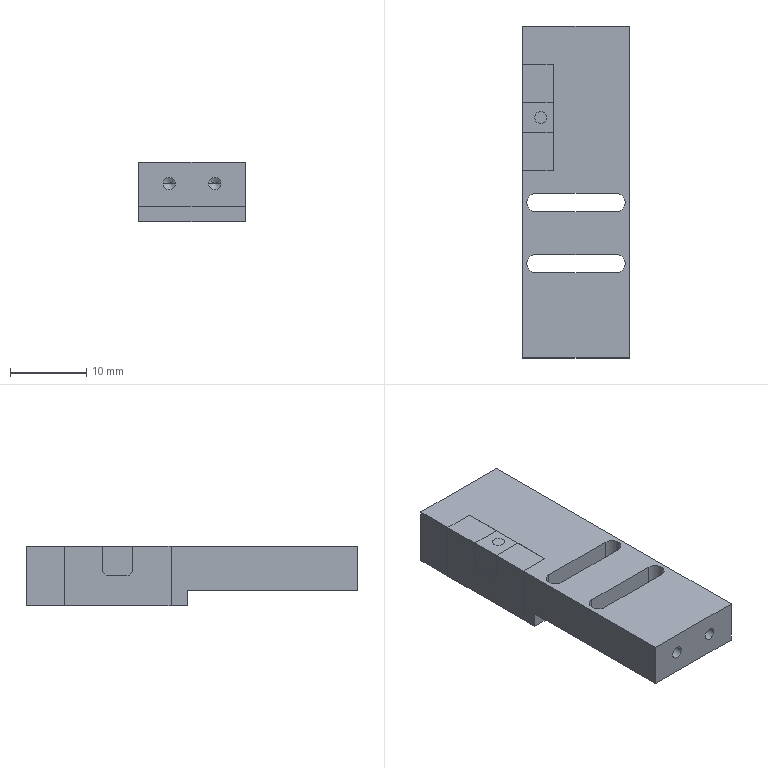NC program | NX | posted with a generic post | part box 14 x 43.5 x 7.8 mm
Whole program:
N10 G17 G21 G94 G90
(DRILLING_COPY_1_COPY , TOOL : D6A45)
N12 T07 M6
N14 G54
N16 G17 G0 G90 X-14.25 Y0.4 B0. C0. S5000 M3
N18 G43 Z30. H7
N20 G94 G81 G98 Z-1. F250. R3.
N22 X-5.25
N24 G80
N26 G0 X-5.25 Y0.4 Z30.
N28 M5
(DRILLING_COPY_COPY_COPY_COPY , TOOL : 1.6ZT)
N30 T14 M6
N32 G54
N34 G17 G0 G90 X-14.25 Y0.4 B0. C0. S2000 M3
N36 G43 Z30. H14
N38 G94 G83 G98 Z-9.681 F150. Q2. R3.
N40 X-5.25
N42 G80
N44 G0 X-5.25 Y0.4 Z30.
N46 M5
(FLOOR_WALL_1_COPY_1 , TOOL : D4)
N48 T04 M6
N50 G54
N52 G17 G0 G90 X-9.75 Y-7.9 B0. C0. S9500 M3
N54 G43 Z30. H4
N56 Z0.61
N58 G94 G1 Z-0.39 F1000.
N60 Y-3.9
N62 X-14.65 F2500.
N64 Y3.9
N66 X-13.85
N68 Y-0.27
N70 X-12.12 Y-2.
N72 X-7.38
N74 X-5.65 Y-0.27
N76 Y3.9
N78 X-4.85
N80 Y-3.9
N82 X-9.75
N84 Y-7.9
N86 Z0.61
N88 G0 Z0.22
N90 G1 Z-0.78 F1000.
N92 Y-3.9
N94 X-14.65 F2500.
N96 Y3.9
N98 X-13.85
N100 Y-0.27
N102 X-12.12 Y-2.
N104 X-7.38
N106 X-5.65 Y-0.27
N108 Y3.9
N110 X-4.85
N112 Y-3.9
N114 X-9.75
N116 Y-7.9
N118 Z0.22
N120 G0 Z-0.17
N122 G1 Z-1.17 F1000.
N124 Y-3.9
N126 X-14.65 F2500.
N128 Y3.9
N130 X-13.85
N132 Y-0.27
N134 X-12.12 Y-2.
N136 X-7.38
N138 X-5.65 Y-0.27
N140 Y3.9
N142 X-4.85
N144 Y-3.9
N146 X-9.75
N148 Y-7.9
N150 Z-0.17
N152 G0 Z-0.56
N154 G1 Z-1.56 F1000.
N156 Y-3.9
N158 X-14.65 F2500.
N160 Y3.9
N162 X-13.85
N164 Y-0.27
N166 X-12.12 Y-2.
N168 X-7.38
N170 X-5.65 Y-0.27
N172 Y3.9
N174 X-4.85
N176 Y-3.9
N178 X-9.75
N180 Y-7.9
N182 Z-0.56
N184 G0 Z-0.95
N186 G1 Z-1.95 F1000.
N188 Y-3.9
N190 X-14.65 F2500.
N192 Y3.9
N194 X-13.85
N196 Y-0.27
N198 X-12.12 Y-2.
N200 X-7.38
N202 X-5.65 Y-0.27
N204 Y3.9
N206 X-4.85
N208 Y-3.9
N210 X-9.75
N212 Y-7.9
N214 Z-0.95
N216 G0 Z-1.34
N218 G1 Z-2.34 F1000.
N220 Y-3.9
N222 X-14.65 F2500.
N224 Y3.9
N226 X-13.85
N228 Y-0.27
N230 X-12.12 Y-2.
N232 X-7.38
N234 X-5.65 Y-0.27
N236 Y3.9
N238 X-4.85
N240 Y-3.9
N242 X-9.75
N244 Y-7.9
N246 Z-1.34
N248 G0 Z-1.73
N250 G1 Z-2.73 F1000.
N252 Y-3.9
N254 X-14.65 F2500.
N256 Y3.9
N258 X-13.85
N260 Y-0.27
N262 X-12.12 Y-2.
N264 X-7.38
N266 X-5.65 Y-0.27
N268 Y3.9
N270 X-4.85
N272 Y-3.9
N274 X-9.75
N276 Y-7.9
N278 Z-1.73
N280 G0 Z-2.12
N282 G1 Z-3.12 F1000.
N284 Y-3.9
N286 X-14.65 F2500.
N288 Y3.9
N290 X-13.85
N292 Y-0.27
N294 X-12.12 Y-2.
N296 X-7.38
N298 X-5.65 Y-0.27
N300 Y3.9
N302 X-4.85
N304 Y-3.9
N306 X-9.75
N308 Y-7.9
N310 Z-2.12
N312 G0 Z-2.51
N314 G1 Z-3.51 F1000.
N316 Y-3.9
N318 X-14.65 F2500.
N320 Y3.9
N322 X-13.85
N324 Y-0.27
N326 X-12.12 Y-2.
N328 X-7.38
N330 X-5.65 Y-0.27
N332 Y3.9
N334 X-4.85
N336 Y-3.9
N338 X-9.75
N340 Y-7.9
N342 Z-2.51
N344 G0 Z-2.9
N346 G1 Z-3.9 F1000.
N348 Y-3.9
N350 X-14.65 F2500.
N352 Y3.9
N354 X-13.85
N356 Y-0.27
N358 X-12.12 Y-2.
N360 X-7.38
N362 X-5.65 Y-0.27
N364 Y3.9
N366 X-4.85
N368 Y-3.9
N370 X-9.75
N372 Y-7.9
N374 Z-2.9
N376 G0 Z30.
(FLOOR_WALL_1_COPY_COPY , TOOL : D4)
N378 X-14.449 Y-8.
N380 Z-3.
N382 G1 Z-4. F1000.
N384 Y-5.9
N386 Y5.9 F1200.
N388 X-14.05
N390 Y-0.27
N392 X-14.053 Y-0.324
N394 X-14.032 Y-0.375
N396 X-13.991 Y-0.411
N398 X-12.569 Y-1.833
N400 Y-5.9
N402 X-10.689
N404 Y-2.2
N406 X-8.81
N408 Y-5.9
N410 X-6.93
N412 Y-1.832
N414 X-5.509 Y-0.411
N416 X-5.468 Y-0.375
N418 X-5.447 Y-0.324
N420 X-5.45 Y-0.27
N422 Y5.9
N424 X-5.05
N426 Y-5.9
N428 Y-8.
N430 Z-3.
N432 G0 X-4.85
N434 G1 Z-4. F1000.
N436 Y-5.9
N438 Y5.9 F1200.
N440 Y8.
N442 X-5.65
N444 Y5.9 F1000.
N446 Y-0.27 F1200.
N448 X-7.38 Y-2.
N450 X-12.12
N452 X-13.85 Y-0.27
N454 Y5.9
N456 Y8.
N458 X-14.65
N460 Y5.9 F1000.
N462 Y-5.9 F1200.
N464 Y-8.
N466 Z-3.
N468 G0 Z30.
N470 M5
(PLANAR_MILL_COPY_1_COPY_COPY_1 , TOOL : D6A45)
N472 T07 M6
N474 G54
N476 G17 G0 G90 X-4.92 Y-1.8 B0. C0. S9500 M3
N478 G43 Z30. H7
N480 Z0.5
N482 G94 G1 Z-1. F1250.
N484 X-4.516 Y-2.5
N486 G3 X-3.65 Y-3. R1.
N488 G1 Y3.
N490 X-6.85
N492 Y0.641
N494 G2 X-7.143 Y-0.066 R1.
N496 G1 X-7.584 Y-0.507
N498 G2 X-8.291 Y-0.8 R1.
N500 G1 X-11.209
N502 G2 X-11.916 Y-0.507 R1.
N504 G1 X-12.357 Y-0.066
N506 G2 X-12.65 Y0.641 R1.
N508 G1 Y3.
N510 X-15.85
N512 Y-3.
N514 X-3.65
N516 G3 X-4.15 Y-2.134 R1.
N518 G1 X-4.85 Y-1.73
N520 Z0.5
N522 G0 Z30.
N524 M5
(CUT_COMP4 , TOOL : D4)
N526 T04 M6
N528 G54
N530 G17 G0 G90 X-4.817 Y-8.048 B0. C0. S9500 M3
N532 G43 Z30. H4
N534 Z-3.
N536 G94 G1 Z-4. F1000.
N538 G41 X-4.8 Y-7.95 D4
N540 Y-3.9
N542 Y3.9 F1200.
N544 Y4.9
N546 G40
N548 X-4.817 Y4.998
N550 X-5.683
N552 G41 X-5.7 Y4.9 F1000.
N554 Y3.9
N556 Y-0.249 F1200.
N558 X-7.401 Y-1.95
N560 X-12.099
N562 X-13.8 Y-0.249
N564 Y3.9
N566 Y4.9
N568 G40
N570 X-13.817 Y4.998
N572 X-14.683
N574 G41 X-14.7 Y4.9 F1000.
N576 Y3.9
N578 Y-3.9 F1200.
N580 Y-7.95
N582 G40
N584 X-14.683 Y-8.048
N586 Z-3.
N588 G0 Z30.
N590 M5
N592 M2